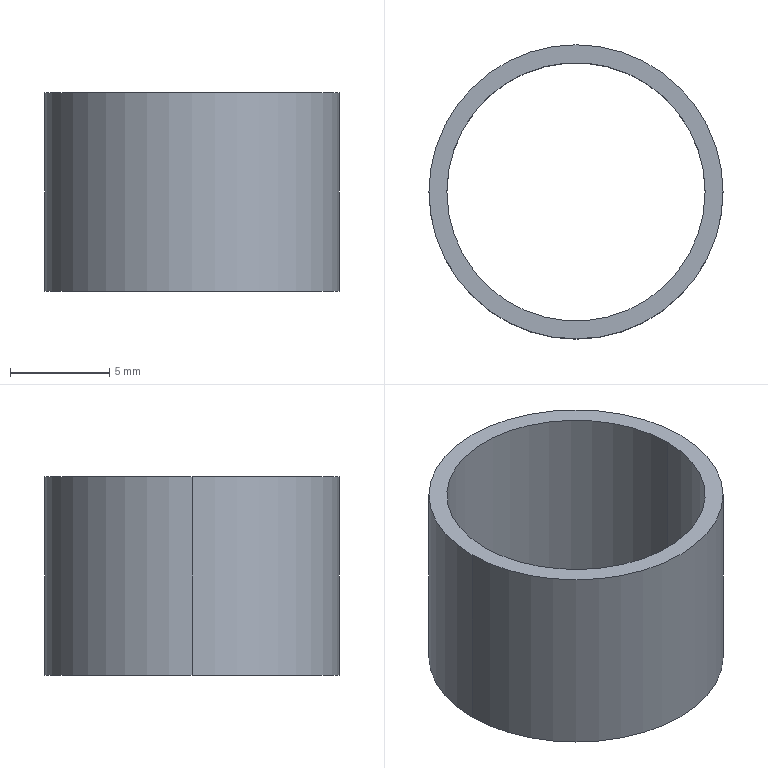Part | SolidWorks | features Extrusion 1 | 1 solid | 6 faces | box 14.8 x 14.8 x 10 mm | volume 393.013 mm3 | cylinder 4 | plane 2 | commonest cylinder face diameters 13 x2 14.8 x2
STEP:
#1=CARTESIAN_POINT('',(-6.5,0.,10.));
#2=VERTEX_POINT('',#1);
#3=CARTESIAN_POINT('',(6.5,0.,10.));
#4=VERTEX_POINT('',#3);
#5=CARTESIAN_POINT('',(0.,0.,10.));
#6=DIRECTION('',(0.,0.,1.));
#7=DIRECTION('',(1.,0.,0.));
#8=AXIS2_PLACEMENT_3D('',#5,#6,#7);
#9=CIRCLE('',#8,6.5);
#10=EDGE_CURVE('',#2,#4,#9,.T.);
#11=ORIENTED_EDGE('',*,*,#10,.T.);
#12=CARTESIAN_POINT('',(6.5,0.,0.));
#13=VERTEX_POINT('',#12);
#14=CARTESIAN_POINT('',(6.5,0.,10.));
#15=DIRECTION('',(0.,0.,-1.));
#16=VECTOR('',#15,1000.);
#17=LINE('',#14,#16);
#18=EDGE_CURVE('',#4,#13,#17,.T.);
#19=ORIENTED_EDGE('',*,*,#18,.T.);
#20=CARTESIAN_POINT('',(-6.5,0.,0.));
#21=VERTEX_POINT('',#20);
#22=CARTESIAN_POINT('',(0.,0.,0.));
#23=DIRECTION('',(0.,0.,1.));
#24=DIRECTION('',(1.,0.,0.));
#25=AXIS2_PLACEMENT_3D('',#22,#23,#24);
#26=CIRCLE('',#25,6.5);
#27=EDGE_CURVE('',#21,#13,#26,.T.);
#28=ORIENTED_EDGE('',*,*,#27,.F.);
#29=CARTESIAN_POINT('',(-6.5,0.,10.));
#30=DIRECTION('',(0.,0.,-1.));
#31=VECTOR('',#30,1000.);
#32=LINE('',#29,#31);
#33=EDGE_CURVE('',#2,#21,#32,.T.);
#34=ORIENTED_EDGE('',*,*,#33,.F.);
#35=EDGE_LOOP('',(#11,#19,#28,#34));
#36=FACE_OUTER_BOUND('',#35,.T.);
#37=CARTESIAN_POINT('',(0.,0.,10.));
#38=DIRECTION('',(0.,0.,-1.));
#39=DIRECTION('',(-1.,0.,0.));
#40=AXIS2_PLACEMENT_3D('',#37,#38,#39);
#41=CYLINDRICAL_SURFACE('',#40,6.5);
#42=ADVANCED_FACE('',(#36),#41,.F.);
#43=CARTESIAN_POINT('',(7.4,0.,10.));
#44=VERTEX_POINT('',#43);
#45=CARTESIAN_POINT('',(-7.4,0.,10.));
#46=VERTEX_POINT('',#45);
#47=CARTESIAN_POINT('',(0.,0.,10.));
#48=DIRECTION('',(0.,0.,1.));
#49=DIRECTION('',(1.,0.,0.));
#50=AXIS2_PLACEMENT_3D('',#47,#48,#49);
#51=CIRCLE('',#50,7.4);
#52=EDGE_CURVE('',#44,#46,#51,.T.);
#53=ORIENTED_EDGE('',*,*,#52,.F.);
#54=CARTESIAN_POINT('',(7.4,0.,0.));
#55=VERTEX_POINT('',#54);
#56=CARTESIAN_POINT('',(7.4,0.,10.));
#57=DIRECTION('',(0.,0.,-1.));
#58=VECTOR('',#57,1000.);
#59=LINE('',#56,#58);
#60=EDGE_CURVE('',#44,#55,#59,.T.);
#61=ORIENTED_EDGE('',*,*,#60,.T.);
#62=CARTESIAN_POINT('',(-7.4,0.,0.));
#63=VERTEX_POINT('',#62);
#64=CARTESIAN_POINT('',(0.,0.,0.));
#65=DIRECTION('',(0.,0.,1.));
#66=DIRECTION('',(1.,0.,0.));
#67=AXIS2_PLACEMENT_3D('',#64,#65,#66);
#68=CIRCLE('',#67,7.4);
#69=EDGE_CURVE('',#55,#63,#68,.T.);
#70=ORIENTED_EDGE('',*,*,#69,.T.);
#71=CARTESIAN_POINT('',(-7.4,0.,10.));
#72=DIRECTION('',(0.,0.,-1.));
#73=VECTOR('',#72,1000.);
#74=LINE('',#71,#73);
#75=EDGE_CURVE('',#46,#63,#74,.T.);
#76=ORIENTED_EDGE('',*,*,#75,.F.);
#77=EDGE_LOOP('',(#53,#61,#70,#76));
#78=FACE_OUTER_BOUND('',#77,.T.);
#79=CARTESIAN_POINT('',(0.,0.,10.));
#80=DIRECTION('',(0.,0.,-1.));
#81=DIRECTION('',(-1.,0.,0.));
#82=AXIS2_PLACEMENT_3D('',#79,#80,#81);
#83=CYLINDRICAL_SURFACE('',#82,7.4);
#84=ADVANCED_FACE('',(#78),#83,.T.);
#85=CARTESIAN_POINT('',(0.,0.,10.));
#86=DIRECTION('',(0.,0.,1.));
#87=DIRECTION('',(1.,0.,0.));
#88=AXIS2_PLACEMENT_3D('',#85,#86,#87);
#89=CIRCLE('',#88,7.4);
#90=EDGE_CURVE('',#46,#44,#89,.T.);
#91=ORIENTED_EDGE('',*,*,#90,.T.);
#92=ORIENTED_EDGE('',*,*,#52,.T.);
#93=EDGE_LOOP('',(#91,#92));
#94=FACE_OUTER_BOUND('',#93,.T.);
#95=ORIENTED_EDGE('',*,*,#10,.F.);
#96=CARTESIAN_POINT('',(0.,0.,10.));
#97=DIRECTION('',(0.,0.,1.));
#98=DIRECTION('',(1.,0.,0.));
#99=AXIS2_PLACEMENT_3D('',#96,#97,#98);
#100=CIRCLE('',#99,6.5);
#101=EDGE_CURVE('',#4,#2,#100,.T.);
#102=ORIENTED_EDGE('',*,*,#101,.F.);
#103=EDGE_LOOP('',(#95,#102));
#104=FACE_BOUND('',#103,.T.);
#105=CARTESIAN_POINT('',(0.,0.,10.));
#106=DIRECTION('',(0.,0.,1.));
#107=DIRECTION('',(1.,0.,0.));
#108=AXIS2_PLACEMENT_3D('',#105,#106,#107);
#109=PLANE('',#108);
#110=ADVANCED_FACE('',(#94,#104),#109,.T.);
#111=CARTESIAN_POINT('',(0.,0.,0.));
#112=DIRECTION('',(0.,0.,1.));
#113=DIRECTION('',(1.,0.,0.));
#114=AXIS2_PLACEMENT_3D('',#111,#112,#113);
#115=CIRCLE('',#114,7.4);
#116=EDGE_CURVE('',#63,#55,#115,.T.);
#117=ORIENTED_EDGE('',*,*,#116,.F.);
#118=ORIENTED_EDGE('',*,*,#69,.F.);
#119=EDGE_LOOP('',(#117,#118));
#120=FACE_OUTER_BOUND('',#119,.T.);
#121=ORIENTED_EDGE('',*,*,#27,.T.);
#122=CARTESIAN_POINT('',(0.,0.,0.));
#123=DIRECTION('',(0.,0.,1.));
#124=DIRECTION('',(1.,0.,0.));
#125=AXIS2_PLACEMENT_3D('',#122,#123,#124);
#126=CIRCLE('',#125,6.5);
#127=EDGE_CURVE('',#13,#21,#126,.T.);
#128=ORIENTED_EDGE('',*,*,#127,.T.);
#129=EDGE_LOOP('',(#121,#128));
#130=FACE_BOUND('',#129,.T.);
#131=CARTESIAN_POINT('',(0.,0.,0.));
#132=DIRECTION('',(0.,0.,1.));
#133=DIRECTION('',(1.,0.,0.));
#134=AXIS2_PLACEMENT_3D('',#131,#132,#133);
#135=PLANE('',#134);
#136=ADVANCED_FACE('',(#120,#130),#135,.F.);
#137=ORIENTED_EDGE('',*,*,#60,.F.);
#138=ORIENTED_EDGE('',*,*,#90,.F.);
#139=ORIENTED_EDGE('',*,*,#75,.T.);
#140=ORIENTED_EDGE('',*,*,#116,.T.);
#141=EDGE_LOOP('',(#137,#138,#139,#140));
#142=FACE_OUTER_BOUND('',#141,.T.);
#143=CARTESIAN_POINT('',(0.,0.,10.));
#144=DIRECTION('',(0.,0.,-1.));
#145=DIRECTION('',(-1.,0.,0.));
#146=AXIS2_PLACEMENT_3D('',#143,#144,#145);
#147=CYLINDRICAL_SURFACE('',#146,7.4);
#148=ADVANCED_FACE('',(#142),#147,.T.);
#149=ORIENTED_EDGE('',*,*,#18,.F.);
#150=ORIENTED_EDGE('',*,*,#101,.T.);
#151=ORIENTED_EDGE('',*,*,#33,.T.);
#152=ORIENTED_EDGE('',*,*,#127,.F.);
#153=EDGE_LOOP('',(#149,#150,#151,#152));
#154=FACE_OUTER_BOUND('',#153,.T.);
#155=CARTESIAN_POINT('',(0.,0.,10.));
#156=DIRECTION('',(0.,0.,-1.));
#157=DIRECTION('',(-1.,0.,0.));
#158=AXIS2_PLACEMENT_3D('',#155,#156,#157);
#159=CYLINDRICAL_SURFACE('',#158,6.5);
#160=ADVANCED_FACE('',(#154),#159,.F.);
#161=CLOSED_SHELL('',(#42,#84,#110,#136,#148,#160));
#162=MANIFOLD_SOLID_BREP('',#161);
#163=CARTESIAN_POINT('',(0.,0.,0.));
#164=DIRECTION('',(0.,0.,1.));
#165=DIRECTION('',(1.,0.,0.));
#166=AXIS2_PLACEMENT_3D('',#163,#164,#165);
#167=(LENGTH_UNIT()NAMED_UNIT(*)SI_UNIT(.MILLI.,.METRE.));
#168=UNCERTAINTY_MEASURE_WITH_UNIT(LENGTH_MEASURE(0.00001),#167,'','');
#169=(NAMED_UNIT(*)PLANE_ANGLE_UNIT()SI_UNIT($,.RADIAN.));
#170=(NAMED_UNIT(*)SI_UNIT($,.STERADIAN.)SOLID_ANGLE_UNIT());
#171=(GEOMETRIC_REPRESENTATION_CONTEXT(3)GLOBAL_UNCERTAINTY_ASSIGNED_CONTEXT((#168))GLOBAL_UNIT_ASSIGNED_CONTEXT((#167,#169,#170))REPRESENTATION_CONTEXT('',''));
#172=ADVANCED_BREP_SHAPE_REPRESENTATION('',(#162,#166),#171);